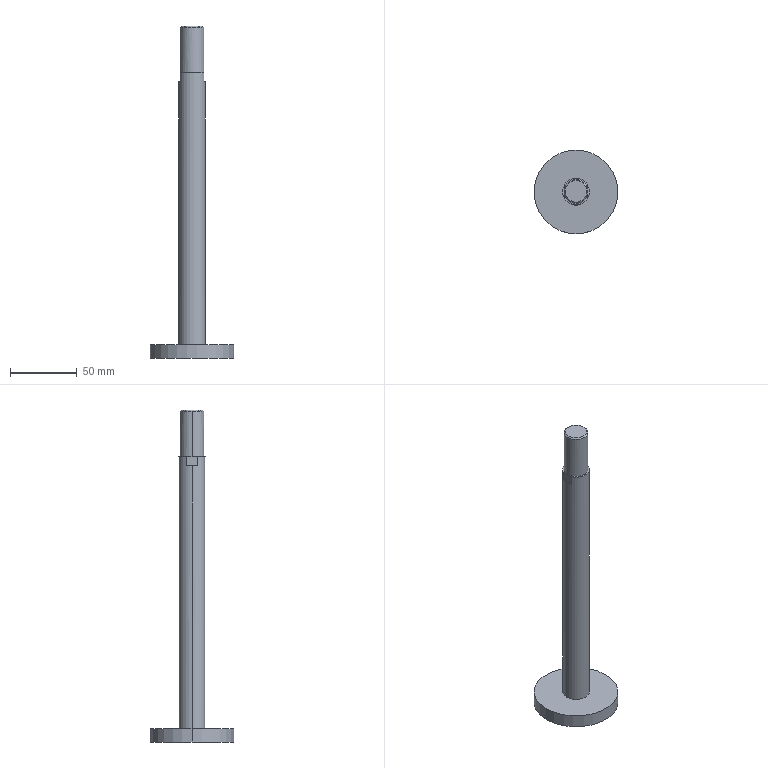Part | SolidWorks | features BaseBody 1 | 1 solid | 17 faces | box 63 x 63 x 249.5 mm | volume 104219 mm3 | plane 9 | cylinder 6 | cone 2 | commonest cylinder face diameters 18 x2 20 x2 63 x2
STEP:
#1=CARTESIAN_POINT('',(9.,4.359,16.));
#2=VERTEX_POINT('',#1);
#3=CARTESIAN_POINT('',(10.,0.,16.));
#4=VERTEX_POINT('',#3);
#5=CARTESIAN_POINT('',(0.,0.,16.));
#6=DIRECTION('',(0.,0.,-1.));
#7=DIRECTION('',(-1.,0.,0.));
#8=AXIS2_PLACEMENT_3D('',#5,#6,#7);
#9=CIRCLE('',#8,10.);
#10=EDGE_CURVE('',#2,#4,#9,.T.);
#11=ORIENTED_EDGE('',*,*,#10,.T.);
#12=CARTESIAN_POINT('',(10.,0.,-181.5));
#13=VERTEX_POINT('',#12);
#14=CARTESIAN_POINT('',(10.,0.,-191.5));
#15=DIRECTION('',(0.,0.,-1.));
#16=VECTOR('',#15,1000.);
#17=LINE('',#14,#16);
#18=EDGE_CURVE('',#4,#13,#17,.T.);
#19=ORIENTED_EDGE('',*,*,#18,.T.);
#20=CARTESIAN_POINT('',(-10.,0.,-181.5));
#21=VERTEX_POINT('',#20);
#22=CARTESIAN_POINT('',(0.,0.,-181.5));
#23=DIRECTION('',(0.,0.,1.));
#24=DIRECTION('',(-1.,0.,0.));
#25=AXIS2_PLACEMENT_3D('',#22,#23,#24);
#26=CIRCLE('',#25,10.);
#27=EDGE_CURVE('',#13,#21,#26,.T.);
#28=ORIENTED_EDGE('',*,*,#27,.T.);
#29=CARTESIAN_POINT('',(-10.,0.,16.));
#30=VERTEX_POINT('',#29);
#31=CARTESIAN_POINT('',(-10.,0.,-191.5));
#32=DIRECTION('',(0.,0.,-1.));
#33=VECTOR('',#32,1000.);
#34=LINE('',#31,#33);
#35=EDGE_CURVE('',#30,#21,#34,.T.);
#36=ORIENTED_EDGE('',*,*,#35,.F.);
#37=CARTESIAN_POINT('',(-9.,4.359,16.));
#38=VERTEX_POINT('',#37);
#39=CARTESIAN_POINT('',(0.,0.,16.));
#40=DIRECTION('',(0.,0.,-1.));
#41=DIRECTION('',(-1.,0.,0.));
#42=AXIS2_PLACEMENT_3D('',#39,#40,#41);
#43=CIRCLE('',#42,10.);
#44=EDGE_CURVE('',#30,#38,#43,.T.);
#45=ORIENTED_EDGE('',*,*,#44,.T.);
#46=CARTESIAN_POINT('',(-9.,4.359,23.));
#47=VERTEX_POINT('',#46);
#48=CARTESIAN_POINT('',(-9.,4.359,-191.5));
#49=DIRECTION('',(0.,0.,1.));
#50=VECTOR('',#49,1000.);
#51=LINE('',#48,#50);
#52=EDGE_CURVE('',#38,#47,#51,.T.);
#53=ORIENTED_EDGE('',*,*,#52,.T.);
#54=CARTESIAN_POINT('',(9.,4.359,23.));
#55=VERTEX_POINT('',#54);
#56=CARTESIAN_POINT('',(0.,0.,23.));
#57=DIRECTION('',(0.,0.,-1.));
#58=DIRECTION('',(-1.,0.,0.));
#59=AXIS2_PLACEMENT_3D('',#56,#57,#58);
#60=CIRCLE('',#59,10.);
#61=EDGE_CURVE('',#47,#55,#60,.T.);
#62=ORIENTED_EDGE('',*,*,#61,.T.);
#63=CARTESIAN_POINT('',(9.,4.359,-191.5));
#64=DIRECTION('',(0.,0.,-1.));
#65=VECTOR('',#64,1000.);
#66=LINE('',#63,#65);
#67=EDGE_CURVE('',#55,#2,#66,.T.);
#68=ORIENTED_EDGE('',*,*,#67,.T.);
#69=EDGE_LOOP('',(#11,#19,#28,#36,#45,#53,#62,#68));
#70=FACE_OUTER_BOUND('',#69,.T.);
#71=CARTESIAN_POINT('',(0.,0.,-191.5));
#72=DIRECTION('',(0.,0.,-1.));
#73=DIRECTION('',(-1.,0.,0.));
#74=AXIS2_PLACEMENT_3D('',#71,#72,#73);
#75=CYLINDRICAL_SURFACE('',#74,10.);
#76=ADVANCED_FACE('',(#70),#75,.T.);
#77=CARTESIAN_POINT('',(0.,9.,57.08));
#78=VERTEX_POINT('',#77);
#79=CARTESIAN_POINT('',(9.,0.,57.08));
#80=VERTEX_POINT('',#79);
#81=CARTESIAN_POINT('',(0.,0.,57.08));
#82=DIRECTION('',(0.,0.,-1.));
#83=DIRECTION('',(-1.,0.,0.));
#84=AXIS2_PLACEMENT_3D('',#81,#82,#83);
#85=CIRCLE('',#84,9.);
#86=EDGE_CURVE('',#78,#80,#85,.T.);
#87=ORIENTED_EDGE('',*,*,#86,.T.);
#88=CARTESIAN_POINT('',(9.,0.,23.));
#89=VERTEX_POINT('',#88);
#90=CARTESIAN_POINT('',(9.,0.,-191.5));
#91=DIRECTION('',(0.,0.,-1.));
#92=VECTOR('',#91,1000.);
#93=LINE('',#90,#92);
#94=EDGE_CURVE('',#80,#89,#93,.T.);
#95=ORIENTED_EDGE('',*,*,#94,.T.);
#96=CARTESIAN_POINT('',(-9.,0.,23.));
#97=VERTEX_POINT('',#96);
#98=CARTESIAN_POINT('',(0.,0.,23.));
#99=DIRECTION('',(0.,0.,1.));
#100=DIRECTION('',(-1.,0.,0.));
#101=AXIS2_PLACEMENT_3D('',#98,#99,#100);
#102=CIRCLE('',#101,9.);
#103=EDGE_CURVE('',#89,#97,#102,.T.);
#104=ORIENTED_EDGE('',*,*,#103,.T.);
#105=CARTESIAN_POINT('',(-9.,0.,57.08));
#106=VERTEX_POINT('',#105);
#107=CARTESIAN_POINT('',(-9.,0.,-191.5));
#108=DIRECTION('',(0.,0.,-1.));
#109=VECTOR('',#108,1000.);
#110=LINE('',#107,#109);
#111=EDGE_CURVE('',#106,#97,#110,.T.);
#112=ORIENTED_EDGE('',*,*,#111,.F.);
#113=CARTESIAN_POINT('',(0.,0.,57.08));
#114=DIRECTION('',(0.,0.,-1.));
#115=DIRECTION('',(-1.,0.,0.));
#116=AXIS2_PLACEMENT_3D('',#113,#114,#115);
#117=CIRCLE('',#116,9.);
#118=EDGE_CURVE('',#106,#78,#117,.T.);
#119=ORIENTED_EDGE('',*,*,#118,.T.);
#120=EDGE_LOOP('',(#87,#95,#104,#112,#119));
#121=FACE_OUTER_BOUND('',#120,.T.);
#122=CARTESIAN_POINT('',(0.,0.,-191.5));
#123=DIRECTION('',(0.,0.,-1.));
#124=DIRECTION('',(-1.,0.,0.));
#125=AXIS2_PLACEMENT_3D('',#122,#123,#124);
#126=CYLINDRICAL_SURFACE('',#125,9.);
#127=ADVANCED_FACE('',(#121),#126,.T.);
#128=CARTESIAN_POINT('',(-31.5,0.,-181.5));
#129=VERTEX_POINT('',#128);
#130=CARTESIAN_POINT('',(31.5,0.,-181.5));
#131=VERTEX_POINT('',#130);
#132=CARTESIAN_POINT('',(0.,0.,-181.5));
#133=DIRECTION('',(0.,0.,-1.));
#134=DIRECTION('',(-1.,0.,0.));
#135=AXIS2_PLACEMENT_3D('',#132,#133,#134);
#136=CIRCLE('',#135,31.5);
#137=EDGE_CURVE('',#129,#131,#136,.T.);
#138=ORIENTED_EDGE('',*,*,#137,.T.);
#139=CARTESIAN_POINT('',(31.5,0.,-191.5));
#140=VERTEX_POINT('',#139);
#141=CARTESIAN_POINT('',(31.5,0.,-191.5));
#142=DIRECTION('',(0.,0.,-1.));
#143=VECTOR('',#142,1000.);
#144=LINE('',#141,#143);
#145=EDGE_CURVE('',#131,#140,#144,.T.);
#146=ORIENTED_EDGE('',*,*,#145,.T.);
#147=CARTESIAN_POINT('',(-31.5,0.,-191.5));
#148=VERTEX_POINT('',#147);
#149=CARTESIAN_POINT('',(0.,0.,-191.5));
#150=DIRECTION('',(0.,0.,1.));
#151=DIRECTION('',(-1.,0.,0.));
#152=AXIS2_PLACEMENT_3D('',#149,#150,#151);
#153=CIRCLE('',#152,31.5);
#154=EDGE_CURVE('',#140,#148,#153,.T.);
#155=ORIENTED_EDGE('',*,*,#154,.T.);
#156=CARTESIAN_POINT('',(-31.5,0.,-191.5));
#157=DIRECTION('',(0.,0.,-1.));
#158=VECTOR('',#157,1000.);
#159=LINE('',#156,#158);
#160=EDGE_CURVE('',#129,#148,#159,.T.);
#161=ORIENTED_EDGE('',*,*,#160,.F.);
#162=EDGE_LOOP('',(#138,#146,#155,#161));
#163=FACE_OUTER_BOUND('',#162,.T.);
#164=CARTESIAN_POINT('',(0.,0.,-191.5));
#165=DIRECTION('',(0.,0.,-1.));
#166=DIRECTION('',(-1.,0.,0.));
#167=AXIS2_PLACEMENT_3D('',#164,#165,#166);
#168=CYLINDRICAL_SURFACE('',#167,31.5);
#169=ADVANCED_FACE('',(#163),#168,.T.);
#170=CARTESIAN_POINT('',(0.,8.08,58.));
#171=VERTEX_POINT('',#170);
#172=CARTESIAN_POINT('',(0.,-8.08,58.));
#173=VERTEX_POINT('',#172);
#174=CARTESIAN_POINT('',(0.,0.,58.));
#175=DIRECTION('',(0.,0.,-1.));
#176=DIRECTION('',(0.,1.,0.));
#177=AXIS2_PLACEMENT_3D('',#174,#175,#176);
#178=CIRCLE('',#177,8.08);
#179=EDGE_CURVE('',#171,#173,#178,.T.);
#180=ORIENTED_EDGE('',*,*,#179,.T.);
#181=CARTESIAN_POINT('',(0.,-9.,57.08));
#182=VERTEX_POINT('',#181);
#183=CARTESIAN_POINT('',(0.,-9.,57.08));
#184=DIRECTION('',(0.,-0.7071,-0.7071));
#185=VECTOR('',#184,1000.);
#186=LINE('',#183,#185);
#187=EDGE_CURVE('',#173,#182,#186,.T.);
#188=ORIENTED_EDGE('',*,*,#187,.T.);
#189=CARTESIAN_POINT('',(0.,0.,57.08));
#190=DIRECTION('',(0.,0.,-1.));
#191=DIRECTION('',(-1.,0.,0.));
#192=AXIS2_PLACEMENT_3D('',#189,#190,#191);
#193=CIRCLE('',#192,9.);
#194=EDGE_CURVE('',#80,#182,#193,.T.);
#195=ORIENTED_EDGE('',*,*,#194,.F.);
#196=ORIENTED_EDGE('',*,*,#86,.F.);
#197=CARTESIAN_POINT('',(0.,9.,57.08));
#198=DIRECTION('',(0.,0.7071,-0.7071));
#199=VECTOR('',#198,1000.);
#200=LINE('',#197,#199);
#201=EDGE_CURVE('',#171,#78,#200,.T.);
#202=ORIENTED_EDGE('',*,*,#201,.F.);
#203=EDGE_LOOP('',(#180,#188,#195,#196,#202));
#204=FACE_OUTER_BOUND('',#203,.T.);
#205=CARTESIAN_POINT('',(0.,0.,57.08));
#206=DIRECTION('',(0.,0.,-1.));
#207=DIRECTION('',(0.,1.,0.));
#208=AXIS2_PLACEMENT_3D('',#205,#206,#207);
#209=CONICAL_SURFACE('',#208,9.,0.7854);
#210=ADVANCED_FACE('',(#204),#209,.T.);
#211=ORIENTED_EDGE('',*,*,#18,.F.);
#212=CARTESIAN_POINT('',(9.,-4.359,16.));
#213=VERTEX_POINT('',#212);
#214=CARTESIAN_POINT('',(0.,0.,16.));
#215=DIRECTION('',(0.,0.,-1.));
#216=DIRECTION('',(-1.,0.,0.));
#217=AXIS2_PLACEMENT_3D('',#214,#215,#216);
#218=CIRCLE('',#217,10.);
#219=EDGE_CURVE('',#4,#213,#218,.T.);
#220=ORIENTED_EDGE('',*,*,#219,.T.);
#221=CARTESIAN_POINT('',(9.,-4.359,23.));
#222=VERTEX_POINT('',#221);
#223=CARTESIAN_POINT('',(9.,-4.359,-191.5));
#224=DIRECTION('',(0.,0.,1.));
#225=VECTOR('',#224,1000.);
#226=LINE('',#223,#225);
#227=EDGE_CURVE('',#213,#222,#226,.T.);
#228=ORIENTED_EDGE('',*,*,#227,.T.);
#229=CARTESIAN_POINT('',(-9.,-4.359,23.));
#230=VERTEX_POINT('',#229);
#231=CARTESIAN_POINT('',(0.,0.,23.));
#232=DIRECTION('',(0.,0.,-1.));
#233=DIRECTION('',(-1.,0.,0.));
#234=AXIS2_PLACEMENT_3D('',#231,#232,#233);
#235=CIRCLE('',#234,10.);
#236=EDGE_CURVE('',#222,#230,#235,.T.);
#237=ORIENTED_EDGE('',*,*,#236,.T.);
#238=CARTESIAN_POINT('',(-9.,-4.359,16.));
#239=VERTEX_POINT('',#238);
#240=CARTESIAN_POINT('',(-9.,-4.359,-191.5));
#241=DIRECTION('',(0.,0.,-1.));
#242=VECTOR('',#241,1000.);
#243=LINE('',#240,#242);
#244=EDGE_CURVE('',#230,#239,#243,.T.);
#245=ORIENTED_EDGE('',*,*,#244,.T.);
#246=CARTESIAN_POINT('',(0.,0.,16.));
#247=DIRECTION('',(0.,0.,-1.));
#248=DIRECTION('',(-1.,0.,0.));
#249=AXIS2_PLACEMENT_3D('',#246,#247,#248);
#250=CIRCLE('',#249,10.);
#251=EDGE_CURVE('',#239,#30,#250,.T.);
#252=ORIENTED_EDGE('',*,*,#251,.T.);
#253=ORIENTED_EDGE('',*,*,#35,.T.);
#254=CARTESIAN_POINT('',(0.,0.,-181.5));
#255=DIRECTION('',(0.,0.,1.));
#256=DIRECTION('',(-1.,0.,0.));
#257=AXIS2_PLACEMENT_3D('',#254,#255,#256);
#258=CIRCLE('',#257,10.);
#259=EDGE_CURVE('',#21,#13,#258,.T.);
#260=ORIENTED_EDGE('',*,*,#259,.T.);
#261=EDGE_LOOP('',(#211,#220,#228,#237,#245,#252,#253,#260));
#262=FACE_OUTER_BOUND('',#261,.T.);
#263=CARTESIAN_POINT('',(0.,0.,-191.5));
#264=DIRECTION('',(0.,0.,-1.));
#265=DIRECTION('',(-1.,0.,0.));
#266=AXIS2_PLACEMENT_3D('',#263,#264,#265);
#267=CYLINDRICAL_SURFACE('',#266,10.);
#268=ADVANCED_FACE('',(#262),#267,.T.);
#269=ORIENTED_EDGE('',*,*,#244,.F.);
#270=CARTESIAN_POINT('',(-9.,4.359,23.));
#271=DIRECTION('',(0.,1.,0.));
#272=VECTOR('',#271,1000.);
#273=LINE('',#270,#272);
#274=EDGE_CURVE('',#230,#97,#273,.T.);
#275=ORIENTED_EDGE('',*,*,#274,.T.);
#276=CARTESIAN_POINT('',(-9.,4.359,23.));
#277=DIRECTION('',(0.,1.,0.));
#278=VECTOR('',#277,1000.);
#279=LINE('',#276,#278);
#280=EDGE_CURVE('',#97,#47,#279,.T.);
#281=ORIENTED_EDGE('',*,*,#280,.T.);
#282=ORIENTED_EDGE('',*,*,#52,.F.);
#283=CARTESIAN_POINT('',(-9.,4.359,16.));
#284=DIRECTION('',(0.,-1.,0.));
#285=VECTOR('',#284,1000.);
#286=LINE('',#283,#285);
#287=EDGE_CURVE('',#38,#239,#286,.T.);
#288=ORIENTED_EDGE('',*,*,#287,.T.);
#289=EDGE_LOOP('',(#269,#275,#281,#282,#288));
#290=FACE_OUTER_BOUND('',#289,.T.);
#291=CARTESIAN_POINT('',(-9.,4.359,16.));
#292=DIRECTION('',(-1.,0.,0.));
#293=DIRECTION('',(0.,0.,1.));
#294=AXIS2_PLACEMENT_3D('',#291,#292,#293);
#295=PLANE('',#294);
#296=ADVANCED_FACE('',(#290),#295,.T.);
#297=CARTESIAN_POINT('',(0.,0.,23.));
#298=DIRECTION('',(0.,0.,1.));
#299=DIRECTION('',(-1.,0.,0.));
#300=AXIS2_PLACEMENT_3D('',#297,#298,#299);
#301=CIRCLE('',#300,9.);
#302=EDGE_CURVE('',#97,#89,#301,.T.);
#303=ORIENTED_EDGE('',*,*,#302,.F.);
#304=ORIENTED_EDGE('',*,*,#274,.F.);
#305=ORIENTED_EDGE('',*,*,#236,.F.);
#306=CARTESIAN_POINT('',(9.,9.,23.));
#307=DIRECTION('',(0.,-1.,0.));
#308=VECTOR('',#307,1000.);
#309=LINE('',#306,#308);
#310=EDGE_CURVE('',#89,#222,#309,.T.);
#311=ORIENTED_EDGE('',*,*,#310,.F.);
#312=EDGE_LOOP('',(#303,#304,#305,#311));
#313=FACE_OUTER_BOUND('',#312,.T.);
#314=CARTESIAN_POINT('',(0.,9.,23.));
#315=DIRECTION('',(0.,0.,-1.));
#316=DIRECTION('',(-1.,0.,0.));
#317=AXIS2_PLACEMENT_3D('',#314,#315,#316);
#318=PLANE('',#317);
#319=ADVANCED_FACE('',(#313),#318,.F.);
#320=ORIENTED_EDGE('',*,*,#67,.F.);
#321=CARTESIAN_POINT('',(9.,-4.359,23.));
#322=DIRECTION('',(0.,-1.,0.));
#323=VECTOR('',#322,1000.);
#324=LINE('',#321,#323);
#325=EDGE_CURVE('',#55,#89,#324,.T.);
#326=ORIENTED_EDGE('',*,*,#325,.T.);
#327=ORIENTED_EDGE('',*,*,#310,.T.);
#328=ORIENTED_EDGE('',*,*,#227,.F.);
#329=CARTESIAN_POINT('',(9.,-4.359,16.));
#330=DIRECTION('',(0.,1.,0.));
#331=VECTOR('',#330,1000.);
#332=LINE('',#329,#331);
#333=EDGE_CURVE('',#213,#2,#332,.T.);
#334=ORIENTED_EDGE('',*,*,#333,.T.);
#335=EDGE_LOOP('',(#320,#326,#327,#328,#334));
#336=FACE_OUTER_BOUND('',#335,.T.);
#337=CARTESIAN_POINT('',(9.,-4.359,16.));
#338=DIRECTION('',(1.,0.,0.));
#339=DIRECTION('',(0.,0.,-1.));
#340=AXIS2_PLACEMENT_3D('',#337,#338,#339);
#341=PLANE('',#340);
#342=ADVANCED_FACE('',(#336),#341,.T.);
#343=ORIENTED_EDGE('',*,*,#10,.F.);
#344=ORIENTED_EDGE('',*,*,#333,.F.);
#345=ORIENTED_EDGE('',*,*,#219,.F.);
#346=EDGE_LOOP('',(#343,#344,#345));
#347=FACE_OUTER_BOUND('',#346,.T.);
#348=CARTESIAN_POINT('',(0.,0.,16.));
#349=DIRECTION('',(0.,0.,1.));
#350=DIRECTION('',(1.,0.,0.));
#351=AXIS2_PLACEMENT_3D('',#348,#349,#350);
#352=PLANE('',#351);
#353=ADVANCED_FACE('',(#347),#352,.T.);
#354=ORIENTED_EDGE('',*,*,#61,.F.);
#355=ORIENTED_EDGE('',*,*,#280,.F.);
#356=ORIENTED_EDGE('',*,*,#103,.F.);
#357=ORIENTED_EDGE('',*,*,#325,.F.);
#358=EDGE_LOOP('',(#354,#355,#356,#357));
#359=FACE_OUTER_BOUND('',#358,.T.);
#360=CARTESIAN_POINT('',(0.,9.,23.));
#361=DIRECTION('',(0.,0.,-1.));
#362=DIRECTION('',(-1.,0.,0.));
#363=AXIS2_PLACEMENT_3D('',#360,#361,#362);
#364=PLANE('',#363);
#365=ADVANCED_FACE('',(#359),#364,.F.);
#366=ORIENTED_EDGE('',*,*,#251,.F.);
#367=ORIENTED_EDGE('',*,*,#287,.F.);
#368=ORIENTED_EDGE('',*,*,#44,.F.);
#369=EDGE_LOOP('',(#366,#367,#368));
#370=FACE_OUTER_BOUND('',#369,.T.);
#371=CARTESIAN_POINT('',(0.,0.,16.));
#372=DIRECTION('',(0.,0.,1.));
#373=DIRECTION('',(1.,0.,0.));
#374=AXIS2_PLACEMENT_3D('',#371,#372,#373);
#375=PLANE('',#374);
#376=ADVANCED_FACE('',(#370),#375,.T.);
#377=ORIENTED_EDGE('',*,*,#259,.F.);
#378=ORIENTED_EDGE('',*,*,#27,.F.);
#379=EDGE_LOOP('',(#377,#378));
#380=FACE_BOUND('',#379,.T.);
#381=ORIENTED_EDGE('',*,*,#137,.F.);
#382=CARTESIAN_POINT('',(0.,0.,-181.5));
#383=DIRECTION('',(0.,0.,-1.));
#384=DIRECTION('',(-1.,0.,0.));
#385=AXIS2_PLACEMENT_3D('',#382,#383,#384);
#386=CIRCLE('',#385,31.5);
#387=EDGE_CURVE('',#131,#129,#386,.T.);
#388=ORIENTED_EDGE('',*,*,#387,.F.);
#389=EDGE_LOOP('',(#381,#388));
#390=FACE_OUTER_BOUND('',#389,.T.);
#391=CARTESIAN_POINT('',(0.,10.,-181.5));
#392=DIRECTION('',(0.,0.,-1.));
#393=DIRECTION('',(-1.,0.,0.));
#394=AXIS2_PLACEMENT_3D('',#391,#392,#393);
#395=PLANE('',#394);
#396=ADVANCED_FACE('',(#380,#390),#395,.F.);
#397=ORIENTED_EDGE('',*,*,#94,.F.);
#398=ORIENTED_EDGE('',*,*,#194,.T.);
#399=CARTESIAN_POINT('',(0.,0.,57.08));
#400=DIRECTION('',(0.,0.,-1.));
#401=DIRECTION('',(-1.,0.,0.));
#402=AXIS2_PLACEMENT_3D('',#399,#400,#401);
#403=CIRCLE('',#402,9.);
#404=EDGE_CURVE('',#182,#106,#403,.T.);
#405=ORIENTED_EDGE('',*,*,#404,.T.);
#406=ORIENTED_EDGE('',*,*,#111,.T.);
#407=ORIENTED_EDGE('',*,*,#302,.T.);
#408=EDGE_LOOP('',(#397,#398,#405,#406,#407));
#409=FACE_OUTER_BOUND('',#408,.T.);
#410=CARTESIAN_POINT('',(0.,0.,-191.5));
#411=DIRECTION('',(0.,0.,-1.));
#412=DIRECTION('',(-1.,0.,0.));
#413=AXIS2_PLACEMENT_3D('',#410,#411,#412);
#414=CYLINDRICAL_SURFACE('',#413,9.);
#415=ADVANCED_FACE('',(#409),#414,.T.);
#416=ORIENTED_EDGE('',*,*,#145,.F.);
#417=ORIENTED_EDGE('',*,*,#387,.T.);
#418=ORIENTED_EDGE('',*,*,#160,.T.);
#419=CARTESIAN_POINT('',(0.,0.,-191.5));
#420=DIRECTION('',(0.,0.,1.));
#421=DIRECTION('',(-1.,0.,0.));
#422=AXIS2_PLACEMENT_3D('',#419,#420,#421);
#423=CIRCLE('',#422,31.5);
#424=EDGE_CURVE('',#148,#140,#423,.T.);
#425=ORIENTED_EDGE('',*,*,#424,.T.);
#426=EDGE_LOOP('',(#416,#417,#418,#425));
#427=FACE_OUTER_BOUND('',#426,.T.);
#428=CARTESIAN_POINT('',(0.,0.,-191.5));
#429=DIRECTION('',(0.,0.,-1.));
#430=DIRECTION('',(-1.,0.,0.));
#431=AXIS2_PLACEMENT_3D('',#428,#429,#430);
#432=CYLINDRICAL_SURFACE('',#431,31.5);
#433=ADVANCED_FACE('',(#427),#432,.T.);
#434=ORIENTED_EDGE('',*,*,#187,.F.);
#435=CARTESIAN_POINT('',(0.,0.,58.));
#436=DIRECTION('',(0.,0.,-1.));
#437=DIRECTION('',(0.,1.,0.));
#438=AXIS2_PLACEMENT_3D('',#435,#436,#437);
#439=CIRCLE('',#438,8.08);
#440=EDGE_CURVE('',#173,#171,#439,.T.);
#441=ORIENTED_EDGE('',*,*,#440,.T.);
#442=ORIENTED_EDGE('',*,*,#201,.T.);
#443=ORIENTED_EDGE('',*,*,#118,.F.);
#444=ORIENTED_EDGE('',*,*,#404,.F.);
#445=EDGE_LOOP('',(#434,#441,#442,#443,#444));
#446=FACE_OUTER_BOUND('',#445,.T.);
#447=CARTESIAN_POINT('',(0.,0.,57.08));
#448=DIRECTION('',(0.,0.,-1.));
#449=DIRECTION('',(0.,1.,0.));
#450=AXIS2_PLACEMENT_3D('',#447,#448,#449);
#451=CONICAL_SURFACE('',#450,9.,0.7854);
#452=ADVANCED_FACE('',(#446),#451,.T.);
#453=ORIENTED_EDGE('',*,*,#424,.F.);
#454=ORIENTED_EDGE('',*,*,#154,.F.);
#455=EDGE_LOOP('',(#453,#454));
#456=FACE_OUTER_BOUND('',#455,.T.);
#457=CARTESIAN_POINT('',(0.,31.5,-191.5));
#458=DIRECTION('',(0.,0.,1.));
#459=DIRECTION('',(1.,0.,0.));
#460=AXIS2_PLACEMENT_3D('',#457,#458,#459);
#461=PLANE('',#460);
#462=ADVANCED_FACE('',(#456),#461,.F.);
#463=ORIENTED_EDGE('',*,*,#179,.F.);
#464=ORIENTED_EDGE('',*,*,#440,.F.);
#465=EDGE_LOOP('',(#463,#464));
#466=FACE_OUTER_BOUND('',#465,.T.);
#467=CARTESIAN_POINT('',(0.,0.,58.));
#468=DIRECTION('',(0.,0.,-1.));
#469=DIRECTION('',(-1.,0.,0.));
#470=AXIS2_PLACEMENT_3D('',#467,#468,#469);
#471=PLANE('',#470);
#472=ADVANCED_FACE('',(#466),#471,.F.);
#473=CLOSED_SHELL('',(#76,#127,#169,#210,#268,#296,#319,#342,#353,#365,#376,#396,#415,#433,#452,#462,#472));
#474=MANIFOLD_SOLID_BREP('',#473);
#475=CARTESIAN_POINT('',(0.,0.,0.));
#476=DIRECTION('',(0.,0.,1.));
#477=DIRECTION('',(1.,0.,0.));
#478=AXIS2_PLACEMENT_3D('',#475,#476,#477);
#479=(LENGTH_UNIT()NAMED_UNIT(*)SI_UNIT(.MILLI.,.METRE.));
#480=UNCERTAINTY_MEASURE_WITH_UNIT(LENGTH_MEASURE(0.00001),#479,'','');
#481=(NAMED_UNIT(*)PLANE_ANGLE_UNIT()SI_UNIT($,.RADIAN.));
#482=(NAMED_UNIT(*)SI_UNIT($,.STERADIAN.)SOLID_ANGLE_UNIT());
#483=(GEOMETRIC_REPRESENTATION_CONTEXT(3)GLOBAL_UNCERTAINTY_ASSIGNED_CONTEXT((#480))GLOBAL_UNIT_ASSIGNED_CONTEXT((#479,#481,#482))REPRESENTATION_CONTEXT('',''));
#484=ADVANCED_BREP_SHAPE_REPRESENTATION('',(#474,#478),#483);